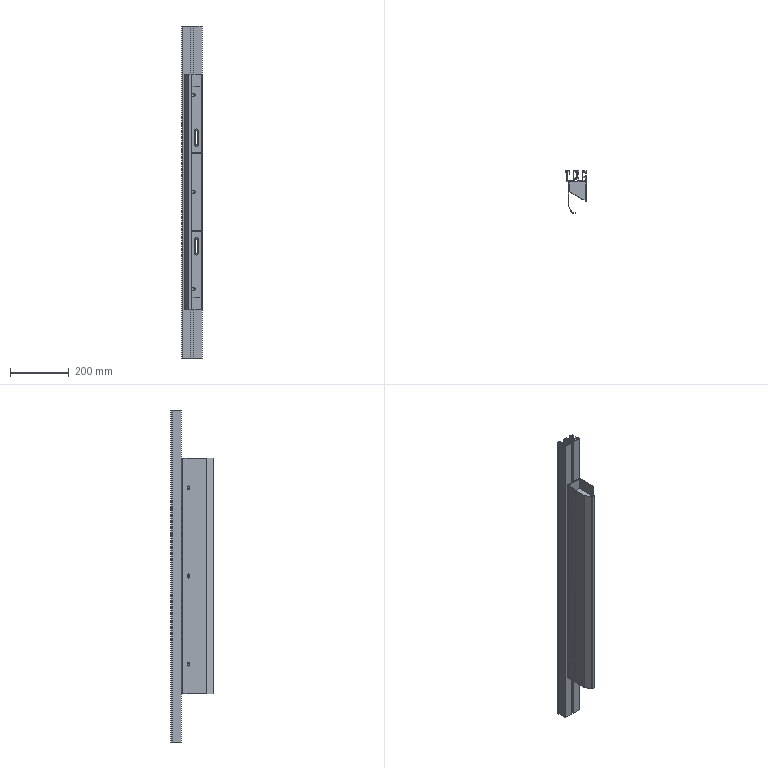Part | SolidWorks | 7 solids | 239 faces | box 70 x 143.651 x 1130 mm | volume 1286253 mm3 | plane 164 | cylinder 75 | commonest cylinder face diameters 10 x19 7 x12 9 x12 2 x8 3 x5 5 x4